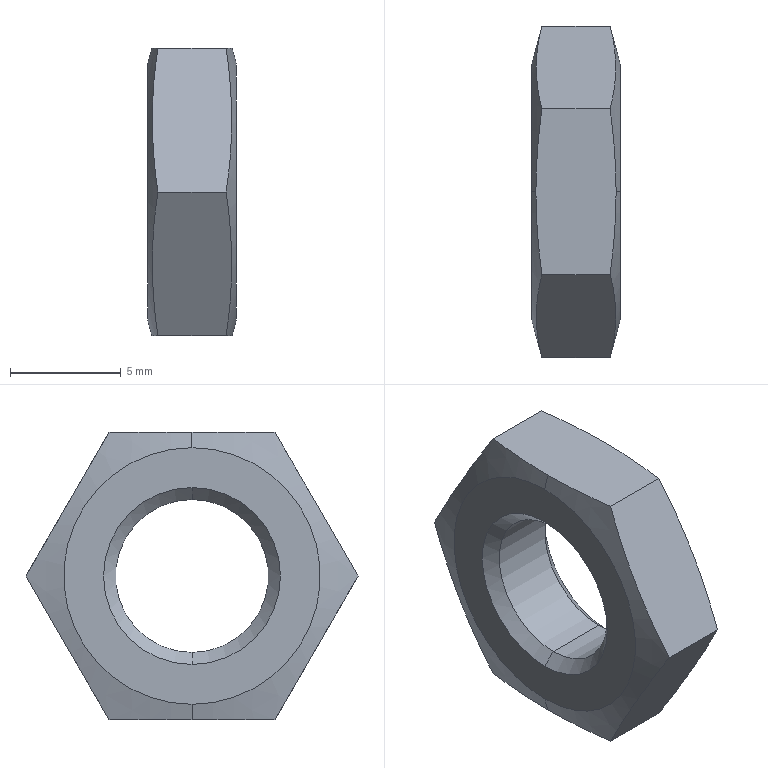Part | NX | features BREP 1 | 1 solid | 18 faces | box 4 x 15.011 x 13 mm | volume 414.842 mm3 | plane 8 | cone 8 | cylinder 2 | commonest cylinder face diameters 6.917 x2
STEP:
#1=CARTESIAN_POINT('',(0.,0.,5.8));
#2=VERTEX_POINT('',#1);
#3=CARTESIAN_POINT('',(0.,0.,-5.8));
#4=VERTEX_POINT('',#3);
#5=CARTESIAN_POINT('',(0.,0.,0.));
#6=DIRECTION('',(1.,0.,0.));
#7=DIRECTION('',(0.,0.,-1.));
#8=AXIS2_PLACEMENT_3D('',#5,#6,#7);
#9=CIRCLE('',#8,5.8);
#10=EDGE_CURVE('',#2,#4,#9,.T.);
#11=ORIENTED_EDGE('',*,*,#10,.F.);
#12=CARTESIAN_POINT('',(0.,0.,0.));
#13=DIRECTION('',(1.,0.,0.));
#14=DIRECTION('',(0.,0.,-1.));
#15=AXIS2_PLACEMENT_3D('',#12,#13,#14);
#16=CIRCLE('',#15,5.8);
#17=EDGE_CURVE('',#4,#2,#16,.T.);
#18=ORIENTED_EDGE('',*,*,#17,.F.);
#19=EDGE_LOOP('',(#11,#18));
#20=FACE_BOUND('',#19,.T.);
#21=CARTESIAN_POINT('',(0.,0.,-4.));
#22=VERTEX_POINT('',#21);
#23=CARTESIAN_POINT('',(0.,0.,4.));
#24=VERTEX_POINT('',#23);
#25=CARTESIAN_POINT('',(0.,0.,0.));
#26=DIRECTION('',(1.,0.,0.));
#27=DIRECTION('',(0.,0.,-1.));
#28=AXIS2_PLACEMENT_3D('',#25,#26,#27);
#29=CIRCLE('',#28,4.);
#30=EDGE_CURVE('',#22,#24,#29,.T.);
#31=ORIENTED_EDGE('',*,*,#30,.T.);
#32=CARTESIAN_POINT('',(0.,0.,0.));
#33=DIRECTION('',(1.,0.,0.));
#34=DIRECTION('',(0.,0.,-1.));
#35=AXIS2_PLACEMENT_3D('',#32,#33,#34);
#36=CIRCLE('',#35,4.);
#37=EDGE_CURVE('',#24,#22,#36,.T.);
#38=ORIENTED_EDGE('',*,*,#37,.T.);
#39=EDGE_LOOP('',(#31,#38));
#40=FACE_BOUND('',#39,.T.);
#41=CARTESIAN_POINT('',(0.,0.,0.));
#42=DIRECTION('',(1.,0.,0.));
#43=DIRECTION('',(0.,0.,1.));
#44=AXIS2_PLACEMENT_3D('',#41,#42,#43);
#45=PLANE('',#44);
#46=ADVANCED_FACE('',(#20,#40),#45,.F.);
#47=CARTESIAN_POINT('',(0.5415,0.,-3.458));
#48=VERTEX_POINT('',#47);
#49=CARTESIAN_POINT('',(0.5415,0.,-3.458));
#50=DIRECTION('',(-0.7071,0.,-0.7071));
#51=VECTOR('',#50,1000.);
#52=LINE('',#49,#51);
#53=EDGE_CURVE('',#48,#22,#52,.T.);
#54=ORIENTED_EDGE('',*,*,#53,.T.);
#55=ORIENTED_EDGE('',*,*,#37,.F.);
#56=CARTESIAN_POINT('',(0.5415,0.,3.458));
#57=VERTEX_POINT('',#56);
#58=CARTESIAN_POINT('',(0.5415,0.,3.458));
#59=DIRECTION('',(-0.7071,0.,0.7071));
#60=VECTOR('',#59,1000.);
#61=LINE('',#58,#60);
#62=EDGE_CURVE('',#57,#24,#61,.T.);
#63=ORIENTED_EDGE('',*,*,#62,.F.);
#64=CARTESIAN_POINT('',(0.5415,0.,0.));
#65=DIRECTION('',(1.,0.,0.));
#66=DIRECTION('',(0.,0.,-1.));
#67=AXIS2_PLACEMENT_3D('',#64,#65,#66);
#68=CIRCLE('',#67,3.458);
#69=EDGE_CURVE('',#57,#48,#68,.T.);
#70=ORIENTED_EDGE('',*,*,#69,.T.);
#71=EDGE_LOOP('',(#54,#55,#63,#70));
#72=FACE_BOUND('',#71,.T.);
#73=CARTESIAN_POINT('',(0.,0.,0.));
#74=DIRECTION('',(-1.,0.,0.));
#75=DIRECTION('',(0.,-1.,0.));
#76=AXIS2_PLACEMENT_3D('',#73,#74,#75);
#77=CONICAL_SURFACE('',#76,4.,0.7854);
#78=ADVANCED_FACE('',(#72),#77,.F.);
#79=CARTESIAN_POINT('',(3.458,0.,3.458));
#80=VERTEX_POINT('',#79);
#81=CARTESIAN_POINT('',(0.5415,0.,3.458));
#82=DIRECTION('',(1.,0.,0.));
#83=VECTOR('',#82,1000.);
#84=LINE('',#81,#83);
#85=EDGE_CURVE('',#80,#57,#84,.F.);
#86=ORIENTED_EDGE('',*,*,#85,.F.);
#87=CARTESIAN_POINT('',(3.458,0.,-3.458));
#88=VERTEX_POINT('',#87);
#89=CARTESIAN_POINT('',(3.458,0.,0.));
#90=DIRECTION('',(1.,0.,0.));
#91=DIRECTION('',(0.,0.,-1.));
#92=AXIS2_PLACEMENT_3D('',#89,#90,#91);
#93=CIRCLE('',#92,3.458);
#94=EDGE_CURVE('',#80,#88,#93,.T.);
#95=ORIENTED_EDGE('',*,*,#94,.T.);
#96=CARTESIAN_POINT('',(0.5415,0.,-3.458));
#97=DIRECTION('',(1.,0.,0.));
#98=VECTOR('',#97,1000.);
#99=LINE('',#96,#98);
#100=EDGE_CURVE('',#88,#48,#99,.F.);
#101=ORIENTED_EDGE('',*,*,#100,.T.);
#102=ORIENTED_EDGE('',*,*,#69,.F.);
#103=EDGE_LOOP('',(#86,#95,#101,#102));
#104=FACE_BOUND('',#103,.T.);
#105=CARTESIAN_POINT('',(4.,0.,0.));
#106=DIRECTION('',(1.,0.,0.));
#107=DIRECTION('',(0.,-1.,0.));
#108=AXIS2_PLACEMENT_3D('',#105,#106,#107);
#109=CYLINDRICAL_SURFACE('',#108,3.458);
#110=ADVANCED_FACE('',(#104),#109,.F.);
#111=ORIENTED_EDGE('',*,*,#85,.T.);
#112=CARTESIAN_POINT('',(0.5415,0.,0.));
#113=DIRECTION('',(1.,0.,0.));
#114=DIRECTION('',(0.,0.,-1.));
#115=AXIS2_PLACEMENT_3D('',#112,#113,#114);
#116=CIRCLE('',#115,3.458);
#117=EDGE_CURVE('',#48,#57,#116,.T.);
#118=ORIENTED_EDGE('',*,*,#117,.F.);
#119=ORIENTED_EDGE('',*,*,#100,.F.);
#120=CARTESIAN_POINT('',(3.458,0.,0.));
#121=DIRECTION('',(1.,0.,0.));
#122=DIRECTION('',(0.,0.,-1.));
#123=AXIS2_PLACEMENT_3D('',#120,#121,#122);
#124=CIRCLE('',#123,3.458);
#125=EDGE_CURVE('',#88,#80,#124,.T.);
#126=ORIENTED_EDGE('',*,*,#125,.T.);
#127=EDGE_LOOP('',(#111,#118,#119,#126));
#128=FACE_BOUND('',#127,.T.);
#129=CARTESIAN_POINT('',(4.,0.,0.));
#130=DIRECTION('',(1.,0.,0.));
#131=DIRECTION('',(0.,1.,0.));
#132=AXIS2_PLACEMENT_3D('',#129,#130,#131);
#133=CYLINDRICAL_SURFACE('',#132,3.458);
#134=ADVANCED_FACE('',(#128),#133,.F.);
#135=CARTESIAN_POINT('',(4.,0.,4.));
#136=VERTEX_POINT('',#135);
#137=CARTESIAN_POINT('',(3.458,0.,3.458));
#138=DIRECTION('',(0.7071,0.,0.7071));
#139=VECTOR('',#138,1000.);
#140=LINE('',#137,#139);
#141=EDGE_CURVE('',#80,#136,#140,.T.);
#142=ORIENTED_EDGE('',*,*,#141,.F.);
#143=ORIENTED_EDGE('',*,*,#125,.F.);
#144=CARTESIAN_POINT('',(4.,0.,-4.));
#145=VERTEX_POINT('',#144);
#146=CARTESIAN_POINT('',(3.458,0.,-3.458));
#147=DIRECTION('',(0.7071,0.,-0.7071));
#148=VECTOR('',#147,1000.);
#149=LINE('',#146,#148);
#150=EDGE_CURVE('',#88,#145,#149,.T.);
#151=ORIENTED_EDGE('',*,*,#150,.T.);
#152=CARTESIAN_POINT('',(4.,0.,0.));
#153=DIRECTION('',(1.,0.,0.));
#154=DIRECTION('',(0.,0.,-1.));
#155=AXIS2_PLACEMENT_3D('',#152,#153,#154);
#156=CIRCLE('',#155,4.);
#157=EDGE_CURVE('',#145,#136,#156,.T.);
#158=ORIENTED_EDGE('',*,*,#157,.T.);
#159=EDGE_LOOP('',(#142,#143,#151,#158));
#160=FACE_BOUND('',#159,.T.);
#161=CARTESIAN_POINT('',(3.458,0.,0.));
#162=DIRECTION('',(1.,0.,0.));
#163=DIRECTION('',(0.,1.,0.));
#164=AXIS2_PLACEMENT_3D('',#161,#162,#163);
#165=CONICAL_SURFACE('',#164,3.458,0.7854);
#166=ADVANCED_FACE('',(#160),#165,.F.);
#167=CARTESIAN_POINT('',(4.,0.,0.));
#168=DIRECTION('',(1.,0.,0.));
#169=DIRECTION('',(0.,0.,-1.));
#170=AXIS2_PLACEMENT_3D('',#167,#168,#169);
#171=CIRCLE('',#170,4.);
#172=EDGE_CURVE('',#136,#145,#171,.T.);
#173=ORIENTED_EDGE('',*,*,#172,.F.);
#174=ORIENTED_EDGE('',*,*,#157,.F.);
#175=EDGE_LOOP('',(#173,#174));
#176=FACE_BOUND('',#175,.T.);
#177=CARTESIAN_POINT('',(4.,0.,-5.8));
#178=VERTEX_POINT('',#177);
#179=CARTESIAN_POINT('',(4.,0.,5.8));
#180=VERTEX_POINT('',#179);
#181=CARTESIAN_POINT('',(4.,0.,0.));
#182=DIRECTION('',(1.,0.,0.));
#183=DIRECTION('',(0.,0.,-1.));
#184=AXIS2_PLACEMENT_3D('',#181,#182,#183);
#185=CIRCLE('',#184,5.8);
#186=EDGE_CURVE('',#178,#180,#185,.T.);
#187=ORIENTED_EDGE('',*,*,#186,.T.);
#188=CARTESIAN_POINT('',(4.,0.,0.));
#189=DIRECTION('',(1.,0.,0.));
#190=DIRECTION('',(0.,0.,-1.));
#191=AXIS2_PLACEMENT_3D('',#188,#189,#190);
#192=CIRCLE('',#191,5.8);
#193=EDGE_CURVE('',#180,#178,#192,.T.);
#194=ORIENTED_EDGE('',*,*,#193,.T.);
#195=EDGE_LOOP('',(#187,#194));
#196=FACE_BOUND('',#195,.T.);
#197=CARTESIAN_POINT('',(4.,5.8,0.));
#198=DIRECTION('',(-1.,0.,0.));
#199=DIRECTION('',(0.,0.,-1.));
#200=AXIS2_PLACEMENT_3D('',#197,#198,#199);
#201=PLANE('',#200);
#202=ADVANCED_FACE('',(#176,#196),#201,.F.);
#203=CARTESIAN_POINT('',(3.812,0.,-6.5));
#204=VERTEX_POINT('',#203);
#205=CARTESIAN_POINT('',(4.,0.,-5.8));
#206=DIRECTION('',(-0.2588,0.,-0.9659));
#207=VECTOR('',#206,1000.);
#208=LINE('',#205,#207);
#209=EDGE_CURVE('',#204,#178,#208,.F.);
#210=ORIENTED_EDGE('',*,*,#209,.T.);
#211=ORIENTED_EDGE('',*,*,#193,.F.);
#212=CARTESIAN_POINT('',(3.812,0.,6.5));
#213=VERTEX_POINT('',#212);
#214=CARTESIAN_POINT('',(4.,0.,5.8));
#215=DIRECTION('',(-0.2588,0.,0.9659));
#216=VECTOR('',#215,1000.);
#217=LINE('',#214,#216);
#218=EDGE_CURVE('',#213,#180,#217,.F.);
#219=ORIENTED_EDGE('',*,*,#218,.F.);
#220=CARTESIAN_POINT('',(3.543,-3.753,6.5));
#221=VERTEX_POINT('',#220);
#222=CARTESIAN_POINT('',(3.812,0.,6.5));
#223=CARTESIAN_POINT('',(3.812,-1.257,6.5));
#224=CARTESIAN_POINT('',(3.71,-2.507,6.5));
#225=CARTESIAN_POINT('',(3.543,-3.753,6.5));
#226=B_SPLINE_CURVE_WITH_KNOTS('',3,(#222,#223,#224,#225),.UNSPECIFIED.,.F.,.F.,(4,4),(0.,0.003762),.UNSPECIFIED.);
#227=EDGE_CURVE('',#213,#221,#226,.T.);
#228=ORIENTED_EDGE('',*,*,#227,.T.);
#229=CARTESIAN_POINT('',(3.543,-7.506,0.));
#230=VERTEX_POINT('',#229);
#231=CARTESIAN_POINT('',(3.543,-3.753,6.5));
#232=CARTESIAN_POINT('',(3.878,-5.004,4.333));
#233=CARTESIAN_POINT('',(3.878,-6.255,2.167));
#234=CARTESIAN_POINT('',(3.543,-7.506,0.));
#235=B_SPLINE_CURVE_WITH_KNOTS('',3,(#231,#232,#233,#234),.UNSPECIFIED.,.F.,.F.,(4,4),(0.,0.007506),.UNSPECIFIED.);
#236=EDGE_CURVE('',#221,#230,#235,.T.);
#237=ORIENTED_EDGE('',*,*,#236,.T.);
#238=CARTESIAN_POINT('',(3.543,-3.753,-6.5));
#239=VERTEX_POINT('',#238);
#240=CARTESIAN_POINT('',(3.543,-7.506,0.));
#241=CARTESIAN_POINT('',(3.878,-6.255,-2.167));
#242=CARTESIAN_POINT('',(3.878,-5.004,-4.333));
#243=CARTESIAN_POINT('',(3.543,-3.753,-6.5));
#244=B_SPLINE_CURVE_WITH_KNOTS('',3,(#240,#241,#242,#243),.UNSPECIFIED.,.F.,.F.,(4,4),(0.,0.007506),.UNSPECIFIED.);
#245=EDGE_CURVE('',#230,#239,#244,.T.);
#246=ORIENTED_EDGE('',*,*,#245,.T.);
#247=CARTESIAN_POINT('',(3.543,-3.753,-6.5));
#248=CARTESIAN_POINT('',(3.71,-2.507,-6.5));
#249=CARTESIAN_POINT('',(3.812,-1.257,-6.5));
#250=CARTESIAN_POINT('',(3.812,0.,-6.5));
#251=B_SPLINE_CURVE_WITH_KNOTS('',3,(#247,#248,#249,#250),.UNSPECIFIED.,.F.,.F.,(4,4),(0.,0.003762),.UNSPECIFIED.);
#252=EDGE_CURVE('',#239,#204,#251,.T.);
#253=ORIENTED_EDGE('',*,*,#252,.T.);
#254=EDGE_LOOP('',(#210,#211,#219,#228,#237,#246,#253));
#255=FACE_BOUND('',#254,.T.);
#256=CARTESIAN_POINT('',(3.464,0.,0.));
#257=DIRECTION('',(-1.,0.,0.));
#258=DIRECTION('',(0.,-1.,0.));
#259=AXIS2_PLACEMENT_3D('',#256,#257,#258);
#260=CONICAL_SURFACE('',#259,7.8,1.309);
#261=ADVANCED_FACE('',(#255),#260,.T.);
#262=CARTESIAN_POINT('',(3.543,3.753,-6.5));
#263=VERTEX_POINT('',#262);
#264=CARTESIAN_POINT('',(0.457,3.753,-6.5));
#265=VERTEX_POINT('',#264);
#266=CARTESIAN_POINT('',(4.,3.753,-6.5));
#267=DIRECTION('',(-1.,0.,0.));
#268=VECTOR('',#267,1000.);
#269=LINE('',#266,#268);
#270=EDGE_CURVE('',#263,#265,#269,.T.);
#271=ORIENTED_EDGE('',*,*,#270,.F.);
#272=CARTESIAN_POINT('',(3.812,0.,-6.5));
#273=CARTESIAN_POINT('',(3.812,1.257,-6.5));
#274=CARTESIAN_POINT('',(3.71,2.507,-6.5));
#275=CARTESIAN_POINT('',(3.543,3.753,-6.5));
#276=B_SPLINE_CURVE_WITH_KNOTS('',3,(#272,#273,#274,#275),.UNSPECIFIED.,.F.,.F.,(4,4),(0.,0.003762),.UNSPECIFIED.);
#277=EDGE_CURVE('',#204,#263,#276,.T.);
#278=ORIENTED_EDGE('',*,*,#277,.F.);
#279=ORIENTED_EDGE('',*,*,#252,.F.);
#280=CARTESIAN_POINT('',(0.457,-3.753,-6.5));
#281=VERTEX_POINT('',#280);
#282=CARTESIAN_POINT('',(4.,-3.753,-6.5));
#283=DIRECTION('',(-1.,0.,0.));
#284=VECTOR('',#283,1000.);
#285=LINE('',#282,#284);
#286=EDGE_CURVE('',#239,#281,#285,.T.);
#287=ORIENTED_EDGE('',*,*,#286,.T.);
#288=CARTESIAN_POINT('',(0.1876,0.,-6.5));
#289=VERTEX_POINT('',#288);
#290=CARTESIAN_POINT('',(0.1876,0.,-6.5));
#291=CARTESIAN_POINT('',(0.1876,-1.257,-6.5));
#292=CARTESIAN_POINT('',(0.2902,-2.507,-6.5));
#293=CARTESIAN_POINT('',(0.457,-3.753,-6.5));
#294=B_SPLINE_CURVE_WITH_KNOTS('',3,(#290,#291,#292,#293),.UNSPECIFIED.,.F.,.F.,(4,4),(0.,0.003762),.UNSPECIFIED.);
#295=EDGE_CURVE('',#289,#281,#294,.T.);
#296=ORIENTED_EDGE('',*,*,#295,.F.);
#297=CARTESIAN_POINT('',(0.457,3.753,-6.5));
#298=CARTESIAN_POINT('',(0.2902,2.507,-6.5));
#299=CARTESIAN_POINT('',(0.1876,1.257,-6.5));
#300=CARTESIAN_POINT('',(0.1876,0.,-6.5));
#301=B_SPLINE_CURVE_WITH_KNOTS('',3,(#297,#298,#299,#300),.UNSPECIFIED.,.F.,.F.,(4,4),(0.,0.003762),.UNSPECIFIED.);
#302=EDGE_CURVE('',#265,#289,#301,.T.);
#303=ORIENTED_EDGE('',*,*,#302,.F.);
#304=EDGE_LOOP('',(#271,#278,#279,#287,#296,#303));
#305=FACE_BOUND('',#304,.T.);
#306=CARTESIAN_POINT('',(4.,-3.753,-6.5));
#307=DIRECTION('',(0.,0.,1.));
#308=DIRECTION('',(-1.,0.,0.));
#309=AXIS2_PLACEMENT_3D('',#306,#307,#308);
#310=PLANE('',#309);
#311=ADVANCED_FACE('',(#305),#310,.F.);
#312=CARTESIAN_POINT('',(0.1876,0.,6.5));
#313=VERTEX_POINT('',#312);
#314=CARTESIAN_POINT('',(0.,0.,5.8));
#315=DIRECTION('',(0.2588,0.,0.9659));
#316=VECTOR('',#315,1000.);
#317=LINE('',#314,#316);
#318=EDGE_CURVE('',#313,#2,#317,.F.);
#319=ORIENTED_EDGE('',*,*,#318,.F.);
#320=CARTESIAN_POINT('',(0.457,3.753,6.5));
#321=VERTEX_POINT('',#320);
#322=CARTESIAN_POINT('',(0.1876,0.,6.5));
#323=CARTESIAN_POINT('',(0.1876,1.257,6.5));
#324=CARTESIAN_POINT('',(0.2902,2.507,6.5));
#325=CARTESIAN_POINT('',(0.457,3.753,6.5));
#326=B_SPLINE_CURVE_WITH_KNOTS('',3,(#322,#323,#324,#325),.UNSPECIFIED.,.F.,.F.,(4,4),(0.,0.003762),.UNSPECIFIED.);
#327=EDGE_CURVE('',#313,#321,#326,.T.);
#328=ORIENTED_EDGE('',*,*,#327,.T.);
#329=CARTESIAN_POINT('',(0.457,7.506,0.));
#330=VERTEX_POINT('',#329);
#331=CARTESIAN_POINT('',(0.457,3.753,6.5));
#332=CARTESIAN_POINT('',(0.1218,5.004,4.333));
#333=CARTESIAN_POINT('',(0.1218,6.255,2.167));
#334=CARTESIAN_POINT('',(0.457,7.506,0.));
#335=B_SPLINE_CURVE_WITH_KNOTS('',3,(#331,#332,#333,#334),.UNSPECIFIED.,.F.,.F.,(4,4),(0.,0.007506),.UNSPECIFIED.);
#336=EDGE_CURVE('',#321,#330,#335,.T.);
#337=ORIENTED_EDGE('',*,*,#336,.T.);
#338=CARTESIAN_POINT('',(0.457,7.506,0.));
#339=CARTESIAN_POINT('',(0.1218,6.255,-2.167));
#340=CARTESIAN_POINT('',(0.1218,5.004,-4.333));
#341=CARTESIAN_POINT('',(0.457,3.753,-6.5));
#342=B_SPLINE_CURVE_WITH_KNOTS('',3,(#338,#339,#340,#341),.UNSPECIFIED.,.F.,.F.,(4,4),(0.,0.007506),.UNSPECIFIED.);
#343=EDGE_CURVE('',#330,#265,#342,.T.);
#344=ORIENTED_EDGE('',*,*,#343,.T.);
#345=ORIENTED_EDGE('',*,*,#302,.T.);
#346=CARTESIAN_POINT('',(0.,0.,-5.8));
#347=DIRECTION('',(0.2588,0.,-0.9659));
#348=VECTOR('',#347,1000.);
#349=LINE('',#346,#348);
#350=EDGE_CURVE('',#289,#4,#349,.F.);
#351=ORIENTED_EDGE('',*,*,#350,.T.);
#352=ORIENTED_EDGE('',*,*,#17,.T.);
#353=EDGE_LOOP('',(#319,#328,#337,#344,#345,#351,#352));
#354=FACE_BOUND('',#353,.T.);
#355=CARTESIAN_POINT('',(0.,0.,0.));
#356=DIRECTION('',(1.,0.,0.));
#357=DIRECTION('',(0.,1.,0.));
#358=AXIS2_PLACEMENT_3D('',#355,#356,#357);
#359=CONICAL_SURFACE('',#358,5.8,1.309);
#360=ADVANCED_FACE('',(#354),#359,.T.);
#361=ORIENTED_EDGE('',*,*,#318,.T.);
#362=ORIENTED_EDGE('',*,*,#10,.T.);
#363=ORIENTED_EDGE('',*,*,#350,.F.);
#364=ORIENTED_EDGE('',*,*,#295,.T.);
#365=CARTESIAN_POINT('',(0.457,-7.506,0.));
#366=VERTEX_POINT('',#365);
#367=CARTESIAN_POINT('',(0.457,-3.753,-6.5));
#368=CARTESIAN_POINT('',(0.1218,-5.004,-4.333));
#369=CARTESIAN_POINT('',(0.1218,-6.255,-2.167));
#370=CARTESIAN_POINT('',(0.457,-7.506,0.));
#371=B_SPLINE_CURVE_WITH_KNOTS('',3,(#367,#368,#369,#370),.UNSPECIFIED.,.F.,.F.,(4,4),(0.,0.007506),.UNSPECIFIED.);
#372=EDGE_CURVE('',#281,#366,#371,.T.);
#373=ORIENTED_EDGE('',*,*,#372,.T.);
#374=CARTESIAN_POINT('',(0.457,-3.753,6.5));
#375=VERTEX_POINT('',#374);
#376=CARTESIAN_POINT('',(0.457,-7.506,0.));
#377=CARTESIAN_POINT('',(0.1218,-6.255,2.167));
#378=CARTESIAN_POINT('',(0.1218,-5.004,4.333));
#379=CARTESIAN_POINT('',(0.457,-3.753,6.5));
#380=B_SPLINE_CURVE_WITH_KNOTS('',3,(#376,#377,#378,#379),.UNSPECIFIED.,.F.,.F.,(4,4),(0.,0.007506),.UNSPECIFIED.);
#381=EDGE_CURVE('',#366,#375,#380,.T.);
#382=ORIENTED_EDGE('',*,*,#381,.T.);
#383=CARTESIAN_POINT('',(0.457,-3.753,6.5));
#384=CARTESIAN_POINT('',(0.2902,-2.507,6.5));
#385=CARTESIAN_POINT('',(0.1876,-1.257,6.5));
#386=CARTESIAN_POINT('',(0.1876,0.,6.5));
#387=B_SPLINE_CURVE_WITH_KNOTS('',3,(#383,#384,#385,#386),.UNSPECIFIED.,.F.,.F.,(4,4),(0.,0.003762),.UNSPECIFIED.);
#388=EDGE_CURVE('',#375,#313,#387,.T.);
#389=ORIENTED_EDGE('',*,*,#388,.T.);
#390=EDGE_LOOP('',(#361,#362,#363,#364,#373,#382,#389));
#391=FACE_BOUND('',#390,.T.);
#392=CARTESIAN_POINT('',(0.,0.,0.));
#393=DIRECTION('',(1.,0.,0.));
#394=DIRECTION('',(0.,-1.,0.));
#395=AXIS2_PLACEMENT_3D('',#392,#393,#394);
#396=CONICAL_SURFACE('',#395,5.8,1.309);
#397=ADVANCED_FACE('',(#391),#396,.T.);
#398=CARTESIAN_POINT('',(4.,-3.753,6.5));
#399=DIRECTION('',(-1.,0.,0.));
#400=VECTOR('',#399,1000.);
#401=LINE('',#398,#400);
#402=EDGE_CURVE('',#221,#375,#401,.T.);
#403=ORIENTED_EDGE('',*,*,#402,.F.);
#404=ORIENTED_EDGE('',*,*,#227,.F.);
#405=CARTESIAN_POINT('',(3.543,3.753,6.5));
#406=VERTEX_POINT('',#405);
#407=CARTESIAN_POINT('',(3.543,3.753,6.5));
#408=CARTESIAN_POINT('',(3.71,2.507,6.5));
#409=CARTESIAN_POINT('',(3.812,1.257,6.5));
#410=CARTESIAN_POINT('',(3.812,0.,6.5));
#411=B_SPLINE_CURVE_WITH_KNOTS('',3,(#407,#408,#409,#410),.UNSPECIFIED.,.F.,.F.,(4,4),(0.,0.003762),.UNSPECIFIED.);
#412=EDGE_CURVE('',#406,#213,#411,.T.);
#413=ORIENTED_EDGE('',*,*,#412,.F.);
#414=CARTESIAN_POINT('',(4.,3.753,6.5));
#415=DIRECTION('',(-1.,0.,0.));
#416=VECTOR('',#415,1000.);
#417=LINE('',#414,#416);
#418=EDGE_CURVE('',#406,#321,#417,.T.);
#419=ORIENTED_EDGE('',*,*,#418,.T.);
#420=ORIENTED_EDGE('',*,*,#327,.F.);
#421=ORIENTED_EDGE('',*,*,#388,.F.);
#422=EDGE_LOOP('',(#403,#404,#413,#419,#420,#421));
#423=FACE_BOUND('',#422,.T.);
#424=CARTESIAN_POINT('',(4.,3.753,6.5));
#425=DIRECTION('',(0.,0.,-1.));
#426=DIRECTION('',(1.,0.,0.));
#427=AXIS2_PLACEMENT_3D('',#424,#425,#426);
#428=PLANE('',#427);
#429=ADVANCED_FACE('',(#423),#428,.F.);
#430=ORIENTED_EDGE('',*,*,#418,.F.);
#431=CARTESIAN_POINT('',(3.543,7.506,0.));
#432=VERTEX_POINT('',#431);
#433=CARTESIAN_POINT('',(3.543,7.506,0.));
#434=CARTESIAN_POINT('',(3.878,6.255,2.167));
#435=CARTESIAN_POINT('',(3.878,5.004,4.333));
#436=CARTESIAN_POINT('',(3.543,3.753,6.5));
#437=B_SPLINE_CURVE_WITH_KNOTS('',3,(#433,#434,#435,#436),.UNSPECIFIED.,.F.,.F.,(4,4),(0.,0.007506),.UNSPECIFIED.);
#438=EDGE_CURVE('',#432,#406,#437,.T.);
#439=ORIENTED_EDGE('',*,*,#438,.F.);
#440=CARTESIAN_POINT('',(4.,7.506,0.));
#441=DIRECTION('',(-1.,0.,0.));
#442=VECTOR('',#441,1000.);
#443=LINE('',#440,#442);
#444=EDGE_CURVE('',#432,#330,#443,.T.);
#445=ORIENTED_EDGE('',*,*,#444,.T.);
#446=ORIENTED_EDGE('',*,*,#336,.F.);
#447=EDGE_LOOP('',(#430,#439,#445,#446));
#448=FACE_BOUND('',#447,.T.);
#449=CARTESIAN_POINT('',(4.,7.506,0.));
#450=DIRECTION('',(0.,-0.866,-0.5));
#451=DIRECTION('',(0.,-0.5,0.866));
#452=AXIS2_PLACEMENT_3D('',#449,#450,#451);
#453=PLANE('',#452);
#454=ADVANCED_FACE('',(#448),#453,.F.);
#455=ORIENTED_EDGE('',*,*,#444,.F.);
#456=CARTESIAN_POINT('',(3.543,3.753,-6.5));
#457=CARTESIAN_POINT('',(3.878,5.004,-4.333));
#458=CARTESIAN_POINT('',(3.878,6.255,-2.167));
#459=CARTESIAN_POINT('',(3.543,7.506,0.));
#460=B_SPLINE_CURVE_WITH_KNOTS('',3,(#456,#457,#458,#459),.UNSPECIFIED.,.F.,.F.,(4,4),(0.,0.007506),.UNSPECIFIED.);
#461=EDGE_CURVE('',#263,#432,#460,.T.);
#462=ORIENTED_EDGE('',*,*,#461,.F.);
#463=ORIENTED_EDGE('',*,*,#270,.T.);
#464=ORIENTED_EDGE('',*,*,#343,.F.);
#465=EDGE_LOOP('',(#455,#462,#463,#464));
#466=FACE_BOUND('',#465,.T.);
#467=CARTESIAN_POINT('',(4.,3.753,-6.5));
#468=DIRECTION('',(0.,-0.866,0.5));
#469=DIRECTION('',(0.,0.5,0.866));
#470=AXIS2_PLACEMENT_3D('',#467,#468,#469);
#471=PLANE('',#470);
#472=ADVANCED_FACE('',(#466),#471,.F.);
#473=ORIENTED_EDGE('',*,*,#209,.F.);
#474=ORIENTED_EDGE('',*,*,#277,.T.);
#475=ORIENTED_EDGE('',*,*,#461,.T.);
#476=ORIENTED_EDGE('',*,*,#438,.T.);
#477=ORIENTED_EDGE('',*,*,#412,.T.);
#478=ORIENTED_EDGE('',*,*,#218,.T.);
#479=ORIENTED_EDGE('',*,*,#186,.F.);
#480=EDGE_LOOP('',(#473,#474,#475,#476,#477,#478,#479));
#481=FACE_BOUND('',#480,.T.);
#482=CARTESIAN_POINT('',(3.464,0.,0.));
#483=DIRECTION('',(-1.,0.,0.));
#484=DIRECTION('',(0.,1.,0.));
#485=AXIS2_PLACEMENT_3D('',#482,#483,#484);
#486=CONICAL_SURFACE('',#485,7.8,1.309);
#487=ADVANCED_FACE('',(#481),#486,.T.);
#488=CARTESIAN_POINT('',(4.,-7.506,0.));
#489=DIRECTION('',(-1.,0.,0.));
#490=VECTOR('',#489,1000.);
#491=LINE('',#488,#490);
#492=EDGE_CURVE('',#230,#366,#491,.T.);
#493=ORIENTED_EDGE('',*,*,#492,.F.);
#494=ORIENTED_EDGE('',*,*,#236,.F.);
#495=ORIENTED_EDGE('',*,*,#402,.T.);
#496=ORIENTED_EDGE('',*,*,#381,.F.);
#497=EDGE_LOOP('',(#493,#494,#495,#496));
#498=FACE_BOUND('',#497,.T.);
#499=CARTESIAN_POINT('',(4.,-3.753,6.5));
#500=DIRECTION('',(0.,0.866,-0.5));
#501=DIRECTION('',(0.,-0.5,-0.866));
#502=AXIS2_PLACEMENT_3D('',#499,#500,#501);
#503=PLANE('',#502);
#504=ADVANCED_FACE('',(#498),#503,.F.);
#505=ORIENTED_EDGE('',*,*,#286,.F.);
#506=ORIENTED_EDGE('',*,*,#245,.F.);
#507=ORIENTED_EDGE('',*,*,#492,.T.);
#508=ORIENTED_EDGE('',*,*,#372,.F.);
#509=EDGE_LOOP('',(#505,#506,#507,#508));
#510=FACE_BOUND('',#509,.T.);
#511=CARTESIAN_POINT('',(4.,-7.506,0.));
#512=DIRECTION('',(0.,0.866,0.5));
#513=DIRECTION('',(0.,0.5,-0.866));
#514=AXIS2_PLACEMENT_3D('',#511,#512,#513);
#515=PLANE('',#514);
#516=ADVANCED_FACE('',(#510),#515,.F.);
#517=ORIENTED_EDGE('',*,*,#141,.T.);
#518=ORIENTED_EDGE('',*,*,#172,.T.);
#519=ORIENTED_EDGE('',*,*,#150,.F.);
#520=ORIENTED_EDGE('',*,*,#94,.F.);
#521=EDGE_LOOP('',(#517,#518,#519,#520));
#522=FACE_BOUND('',#521,.T.);
#523=CARTESIAN_POINT('',(3.458,0.,0.));
#524=DIRECTION('',(1.,0.,0.));
#525=DIRECTION('',(0.,-1.,0.));
#526=AXIS2_PLACEMENT_3D('',#523,#524,#525);
#527=CONICAL_SURFACE('',#526,3.458,0.7854);
#528=ADVANCED_FACE('',(#522),#527,.F.);
#529=ORIENTED_EDGE('',*,*,#53,.F.);
#530=ORIENTED_EDGE('',*,*,#117,.T.);
#531=ORIENTED_EDGE('',*,*,#62,.T.);
#532=ORIENTED_EDGE('',*,*,#30,.F.);
#533=EDGE_LOOP('',(#529,#530,#531,#532));
#534=FACE_BOUND('',#533,.T.);
#535=CARTESIAN_POINT('',(0.,0.,0.));
#536=DIRECTION('',(-1.,0.,0.));
#537=DIRECTION('',(0.,1.,0.));
#538=AXIS2_PLACEMENT_3D('',#535,#536,#537);
#539=CONICAL_SURFACE('',#538,4.,0.7854);
#540=ADVANCED_FACE('',(#534),#539,.F.);
#541=CLOSED_SHELL('',(#46,#78,#110,#134,#166,#202,#261,#311,#360,#397,#429,#454,#472,#487,#504,#516,#528,#540));
#542=MANIFOLD_SOLID_BREP('',#541);
#543=(LENGTH_UNIT()NAMED_UNIT(*)SI_UNIT(.MILLI.,.METRE.));
#544=UNCERTAINTY_MEASURE_WITH_UNIT(LENGTH_MEASURE(0.0508),#543,'','');
#545=(NAMED_UNIT(*)PLANE_ANGLE_UNIT()SI_UNIT($,.RADIAN.));
#546=(NAMED_UNIT(*)SI_UNIT($,.STERADIAN.)SOLID_ANGLE_UNIT());
#547=(GEOMETRIC_REPRESENTATION_CONTEXT(3)GLOBAL_UNCERTAINTY_ASSIGNED_CONTEXT((#544))GLOBAL_UNIT_ASSIGNED_CONTEXT((#543,#545,#546))REPRESENTATION_CONTEXT('',''));
#548=ADVANCED_BREP_SHAPE_REPRESENTATION('',(#542),#547);